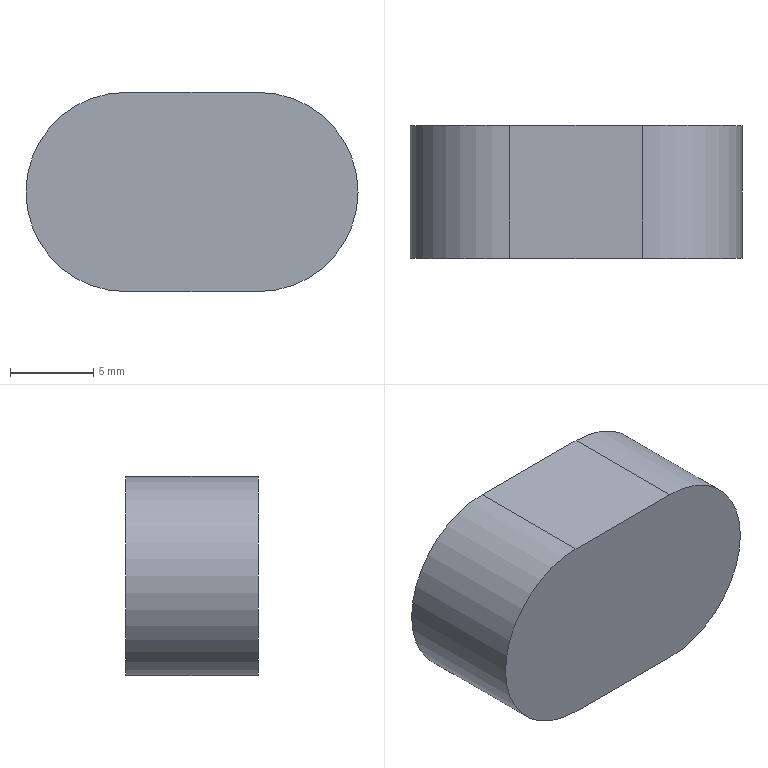Part | SolidWorks | features Extrusion 1 | 1 solid | 6 faces | box 20 x 8 x 12 mm | volume 1673 mm3 | plane 4 | cylinder 2 | commonest cylinder face diameters 12 x2
STEP:
#1=CARTESIAN_POINT('',(-4.,0.,-6.));
#2=VERTEX_POINT('',#1);
#3=CARTESIAN_POINT('',(-4.,0.,6.));
#4=VERTEX_POINT('',#3);
#5=CARTESIAN_POINT('',(-4.,0.,0.));
#6=DIRECTION('',(0.,1.,0.));
#7=DIRECTION('',(0.,0.,1.));
#8=AXIS2_PLACEMENT_3D('',#5,#6,#7);
#9=CIRCLE('',#8,6.);
#10=EDGE_CURVE('',#2,#4,#9,.T.);
#11=ORIENTED_EDGE('',*,*,#10,.T.);
#12=CARTESIAN_POINT('',(-4.,8.,6.));
#13=VERTEX_POINT('',#12);
#14=CARTESIAN_POINT('',(-4.,8.,6.));
#15=DIRECTION('',(0.,-1.,0.));
#16=VECTOR('',#15,1000.);
#17=LINE('',#14,#16);
#18=EDGE_CURVE('',#13,#4,#17,.T.);
#19=ORIENTED_EDGE('',*,*,#18,.F.);
#20=CARTESIAN_POINT('',(-4.,8.,-6.));
#21=VERTEX_POINT('',#20);
#22=CARTESIAN_POINT('',(-4.,8.,0.));
#23=DIRECTION('',(0.,1.,0.));
#24=DIRECTION('',(0.,0.,1.));
#25=AXIS2_PLACEMENT_3D('',#22,#23,#24);
#26=CIRCLE('',#25,6.);
#27=EDGE_CURVE('',#21,#13,#26,.T.);
#28=ORIENTED_EDGE('',*,*,#27,.F.);
#29=CARTESIAN_POINT('',(-4.,8.,-6.));
#30=DIRECTION('',(0.,-1.,0.));
#31=VECTOR('',#30,1000.);
#32=LINE('',#29,#31);
#33=EDGE_CURVE('',#21,#2,#32,.T.);
#34=ORIENTED_EDGE('',*,*,#33,.T.);
#35=EDGE_LOOP('',(#11,#19,#28,#34));
#36=FACE_OUTER_BOUND('',#35,.T.);
#37=CARTESIAN_POINT('',(-4.,8.,0.));
#38=DIRECTION('',(0.,-1.,0.));
#39=DIRECTION('',(0.,0.,-1.));
#40=AXIS2_PLACEMENT_3D('',#37,#38,#39);
#41=CYLINDRICAL_SURFACE('',#40,6.);
#42=ADVANCED_FACE('',(#36),#41,.T.);
#43=CARTESIAN_POINT('',(4.,0.,6.));
#44=VERTEX_POINT('',#43);
#45=CARTESIAN_POINT('',(-4.,0.,6.));
#46=DIRECTION('',(1.,0.,0.));
#47=VECTOR('',#46,1000.);
#48=LINE('',#45,#47);
#49=EDGE_CURVE('',#4,#44,#48,.T.);
#50=ORIENTED_EDGE('',*,*,#49,.T.);
#51=CARTESIAN_POINT('',(4.,8.,6.));
#52=VERTEX_POINT('',#51);
#53=CARTESIAN_POINT('',(4.,8.,6.));
#54=DIRECTION('',(0.,-1.,0.));
#55=VECTOR('',#54,1000.);
#56=LINE('',#53,#55);
#57=EDGE_CURVE('',#52,#44,#56,.T.);
#58=ORIENTED_EDGE('',*,*,#57,.F.);
#59=CARTESIAN_POINT('',(-4.,8.,6.));
#60=DIRECTION('',(1.,0.,0.));
#61=VECTOR('',#60,1000.);
#62=LINE('',#59,#61);
#63=EDGE_CURVE('',#13,#52,#62,.T.);
#64=ORIENTED_EDGE('',*,*,#63,.F.);
#65=ORIENTED_EDGE('',*,*,#18,.T.);
#66=EDGE_LOOP('',(#50,#58,#64,#65));
#67=FACE_OUTER_BOUND('',#66,.T.);
#68=CARTESIAN_POINT('',(-4.,8.,6.));
#69=DIRECTION('',(0.,0.,-1.));
#70=DIRECTION('',(-1.,0.,0.));
#71=AXIS2_PLACEMENT_3D('',#68,#69,#70);
#72=PLANE('',#71);
#73=ADVANCED_FACE('',(#67),#72,.F.);
#74=CARTESIAN_POINT('',(4.,0.,-6.));
#75=VERTEX_POINT('',#74);
#76=CARTESIAN_POINT('',(4.,0.,0.));
#77=DIRECTION('',(0.,1.,0.));
#78=DIRECTION('',(0.,0.,1.));
#79=AXIS2_PLACEMENT_3D('',#76,#77,#78);
#80=CIRCLE('',#79,6.);
#81=EDGE_CURVE('',#44,#75,#80,.T.);
#82=ORIENTED_EDGE('',*,*,#81,.T.);
#83=CARTESIAN_POINT('',(4.,8.,-6.));
#84=VERTEX_POINT('',#83);
#85=CARTESIAN_POINT('',(4.,8.,-6.));
#86=DIRECTION('',(0.,-1.,0.));
#87=VECTOR('',#86,1000.);
#88=LINE('',#85,#87);
#89=EDGE_CURVE('',#84,#75,#88,.T.);
#90=ORIENTED_EDGE('',*,*,#89,.F.);
#91=CARTESIAN_POINT('',(4.,8.,0.));
#92=DIRECTION('',(0.,1.,0.));
#93=DIRECTION('',(0.,0.,1.));
#94=AXIS2_PLACEMENT_3D('',#91,#92,#93);
#95=CIRCLE('',#94,6.);
#96=EDGE_CURVE('',#52,#84,#95,.T.);
#97=ORIENTED_EDGE('',*,*,#96,.F.);
#98=ORIENTED_EDGE('',*,*,#57,.T.);
#99=EDGE_LOOP('',(#82,#90,#97,#98));
#100=FACE_OUTER_BOUND('',#99,.T.);
#101=CARTESIAN_POINT('',(4.,8.,0.));
#102=DIRECTION('',(0.,-1.,0.));
#103=DIRECTION('',(0.,0.,-1.));
#104=AXIS2_PLACEMENT_3D('',#101,#102,#103);
#105=CYLINDRICAL_SURFACE('',#104,6.);
#106=ADVANCED_FACE('',(#100),#105,.T.);
#107=CARTESIAN_POINT('',(-4.,0.,-6.));
#108=DIRECTION('',(-1.,0.,0.));
#109=VECTOR('',#108,1000.);
#110=LINE('',#107,#109);
#111=EDGE_CURVE('',#75,#2,#110,.T.);
#112=ORIENTED_EDGE('',*,*,#111,.T.);
#113=ORIENTED_EDGE('',*,*,#33,.F.);
#114=CARTESIAN_POINT('',(-4.,8.,-6.));
#115=DIRECTION('',(-1.,0.,0.));
#116=VECTOR('',#115,1000.);
#117=LINE('',#114,#116);
#118=EDGE_CURVE('',#84,#21,#117,.T.);
#119=ORIENTED_EDGE('',*,*,#118,.F.);
#120=ORIENTED_EDGE('',*,*,#89,.T.);
#121=EDGE_LOOP('',(#112,#113,#119,#120));
#122=FACE_OUTER_BOUND('',#121,.T.);
#123=CARTESIAN_POINT('',(-4.,8.,-6.));
#124=DIRECTION('',(0.,0.,1.));
#125=DIRECTION('',(1.,0.,0.));
#126=AXIS2_PLACEMENT_3D('',#123,#124,#125);
#127=PLANE('',#126);
#128=ADVANCED_FACE('',(#122),#127,.F.);
#129=ORIENTED_EDGE('',*,*,#27,.T.);
#130=ORIENTED_EDGE('',*,*,#63,.T.);
#131=ORIENTED_EDGE('',*,*,#96,.T.);
#132=ORIENTED_EDGE('',*,*,#118,.T.);
#133=EDGE_LOOP('',(#129,#130,#131,#132));
#134=FACE_OUTER_BOUND('',#133,.T.);
#135=CARTESIAN_POINT('',(-4.,8.,0.));
#136=DIRECTION('',(0.,1.,0.));
#137=DIRECTION('',(0.,0.,1.));
#138=AXIS2_PLACEMENT_3D('',#135,#136,#137);
#139=PLANE('',#138);
#140=ADVANCED_FACE('',(#134),#139,.T.);
#141=ORIENTED_EDGE('',*,*,#10,.F.);
#142=ORIENTED_EDGE('',*,*,#111,.F.);
#143=ORIENTED_EDGE('',*,*,#81,.F.);
#144=ORIENTED_EDGE('',*,*,#49,.F.);
#145=EDGE_LOOP('',(#141,#142,#143,#144));
#146=FACE_OUTER_BOUND('',#145,.T.);
#147=CARTESIAN_POINT('',(-4.,0.,0.));
#148=DIRECTION('',(0.,1.,0.));
#149=DIRECTION('',(0.,0.,1.));
#150=AXIS2_PLACEMENT_3D('',#147,#148,#149);
#151=PLANE('',#150);
#152=ADVANCED_FACE('',(#146),#151,.F.);
#153=CLOSED_SHELL('',(#42,#73,#106,#128,#140,#152));
#154=MANIFOLD_SOLID_BREP('',#153);
#155=CARTESIAN_POINT('',(0.,0.,0.));
#156=DIRECTION('',(0.,0.,1.));
#157=DIRECTION('',(1.,0.,0.));
#158=AXIS2_PLACEMENT_3D('',#155,#156,#157);
#159=(LENGTH_UNIT()NAMED_UNIT(*)SI_UNIT(.MILLI.,.METRE.));
#160=UNCERTAINTY_MEASURE_WITH_UNIT(LENGTH_MEASURE(0.00001),#159,'','');
#161=(NAMED_UNIT(*)PLANE_ANGLE_UNIT()SI_UNIT($,.RADIAN.));
#162=(NAMED_UNIT(*)SI_UNIT($,.STERADIAN.)SOLID_ANGLE_UNIT());
#163=(GEOMETRIC_REPRESENTATION_CONTEXT(3)GLOBAL_UNCERTAINTY_ASSIGNED_CONTEXT((#160))GLOBAL_UNIT_ASSIGNED_CONTEXT((#159,#161,#162))REPRESENTATION_CONTEXT('',''));
#164=ADVANCED_BREP_SHAPE_REPRESENTATION('',(#154,#158),#163);